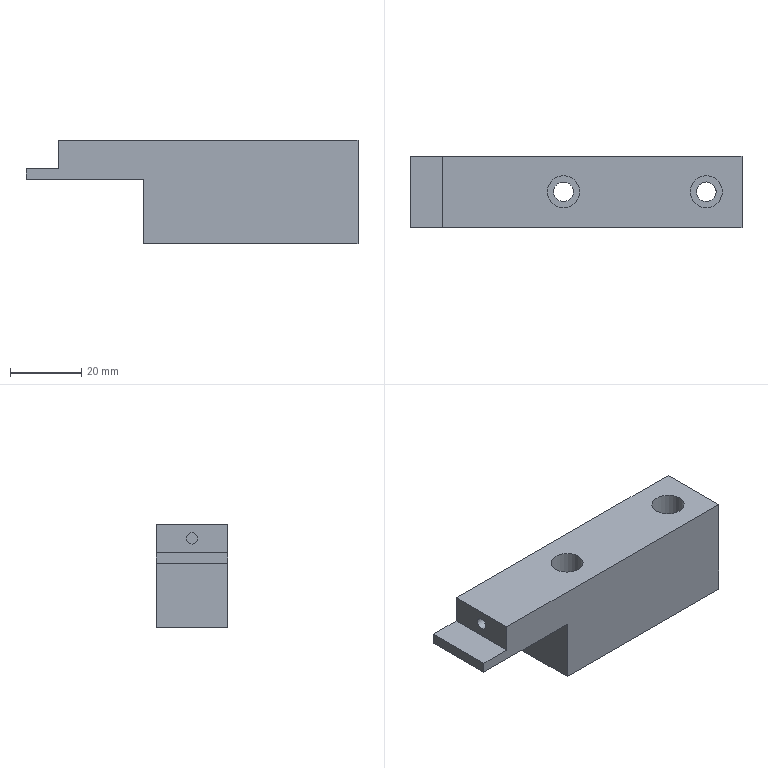CAM job | NX | 3-axis milling, drilling | part box 93 x 20 x 29 mm | stock box 98 x 25 x 35 mm
Tools:
number,name,description,diameter,corner_radius,flute_length,length,flutes
4,D4,平底铣刀-粗,4.0,0.0,25.0,75.0,2
9,D10,平底铣刀-粗,10.0,0.0,35.0,75.0,2
10,D10-J,平底铣刀-精,10.0,0.0,35.0,75.0,2
1,D80R0.8飞刀,圆鼻刀-粗,80.0,0.8,50.0,75.0,2
1,D80R0.8飞刀-J,圆鼻刀-精,80.0,0.8,50.0,75.0,2
2,D6倒角刀,倒角刀,6.0,0.0,3.0,25.0,2
17,钻头5.5,Twist Drill 5 mm,5.5,0.0,52.0,54.0,2
Operations:
program,operation,operation_type,tool,method,geometry_group,spindle_rpm,surface_speed,feed_per_tooth,feed_cut,feed_plunge,cut_length_mm,path_length_mm,cut_time_min,machine_time_min
B,底壁铣飞面一刀开粗_COPY,VolumeBased25DMillingOperation,D80R0.8飞刀,分层开粗-切深K-步距G,W-B,5000.0,1256.637,0.3,3000.0,100.0,1810.746,3586.966,0.6036,0.7812
B,底壁铣飞面一刀精光_COPY,VolumeBased25DMillingOperation,D80R0.8飞刀-J,侧刃精光-切深K-步距G,W-B,5000.0,1256.637,0.1,1000.0,100.0,200.998,236.998,0.201,0.2046
B,底壁铣分层开粗-中_COPY,VolumeBased25DMillingOperation,D10,分层开粗-切深K-步距G,W-B,8000.0,251.32,0.25,4000.0,100.0,5582.289,6990.708,1.396,1.536
B,平面去毛刺6X45L_COPY,SurfaceContour,D6倒角刀,爬面_倒角-切深0-步距G,W-B,6500.0,122.519,0.1154,1500.0,100.0,317.614,530.176,0.2117,0.233
B,底壁铣精光底面-中_COPY,VolumeBased25DMillingOperation,D10-J,精光步距切深关,W-B,6000.0,188.496,0.0833,1000.0,100.0,242.99,307.59,0.243,0.2494
B,底壁铣精光侧面-中-选底面_COPY,VolumeBased25DMillingOperation,D10-J,侧刃精光-切深K-步距G,W-B,6000.0,188.496,0.0833,1000.0,100.0,38.682,104.282,0.0387,0.0452
A,顶面,FaceMilling,D80R0.8飞刀,侧刃精光-切深K-步距G,W-A,5000.0,1256.637,0.1,1000.0,100.0,187.0,223.0,0.187,0.1906
A,外形粗_2,VolumeBased25DMillingOperation,D10,METHOD,W-A,8000.0,251.327,0.3125,5000.0,80.0,10065.271,10133.271,2.013,2.02
A,底壁粗_1,VolumeBased25DMillingOperation,D10,METHOD,W-A,6000.0,113.0,0.2083,3500.0,100.0,1000.0,1174.686,0.2857,0.3032
A,沉头孔打点-深0.8,Operation,D6倒角刀,NONE,W-A,8000.0,150.796,0.0312,500.0,90.0,3.6,88.213,0.0072,0.0157
A,沉头孔-钻孔0段,Operation,钻头5.5,NONE,W-A,2800.0,48.38,0.0357,200.0,90.0,67.305,215.622,0.3365,0.3514
A,铣孔开粗D4_1,CylinderMilling,D4,NONE,W-A,8000.0,100.531,0.075,1200.0,100.0,1651.848,1811.848,1.377,1.393
A,铣孔精光D4_1,CylinderMilling,D4,精光步距切深关,W-A,8000.0,100.531,0.0312,500.0,100.0,116.265,255.265,0.2325,0.2464
A,仅选体,SurfaceContour,D6倒角刀,METHOD,W-A,8000.0,150.796,0.1875,3000.0,100.0,285.077,408.715,0.095,0.1074
A,铣倒角_1,PlanarMilling,D6倒角刀,NONE,W-A,8000.0,150.796,0.0312,500.0,100.0,74.219,179.451,0.1484,0.159
A,底侧精_3,VolumeBased25DMillingOperation,D10-J,METHOD,W-A,6000.0,113.0,0.2083,1200.0,100.0,33.342,88.242,0.0278,0.0333
A,外形半精_2,VolumeBased25DMillingOperation,D10-J,METHOD,W-A,8000.0,251.327,0.0625,1000.0,100.0,524.748,693.763,0.5247,0.5416